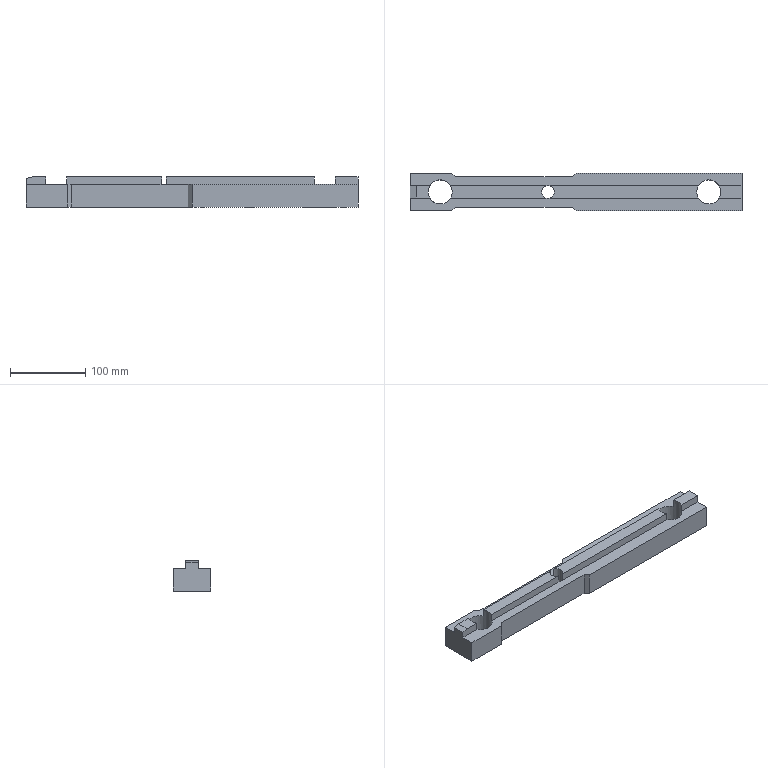Part | STEP file | lll_id3862_x_t | 1 solid | 45 faces | box 440 x 50 x 40 mm | volume 602620 mm3 | plane 31 | cylinder 10 | cone 4 | commonest cylinder face diameters 6.806 x4 11 x2 32 x2 17 x1 22 x1
STEP:
#1=CARTESIAN_POINT('',(2899.856,8.,0.));
#2=VERTEX_POINT('',#1);
#3=CARTESIAN_POINT('',(2899.856,8.,-10.));
#4=VERTEX_POINT('',#3);
#5=CARTESIAN_POINT('',(2899.856,8.,-5.));
#6=DIRECTION('',(0.,0.,-1.));
#7=VECTOR('',#6,1.);
#8=LINE('',#5,#7);
#9=EDGE_CURVE('',#2,#4,#8,.T.);
#10=ORIENTED_EDGE('',*,*,#9,.F.);
#11=CARTESIAN_POINT('',(2930.,8.,0.));
#12=VERTEX_POINT('',#11);
#13=CARTESIAN_POINT('',(2772.5,8.,0.));
#14=DIRECTION('',(1.,0.,0.));
#15=VECTOR('',#14,1.);
#16=LINE('',#13,#15);
#17=EDGE_CURVE('',#2,#12,#16,.T.);
#18=ORIENTED_EDGE('',*,*,#17,.T.);
#19=CARTESIAN_POINT('',(2930.,8.,-10.));
#20=VERTEX_POINT('',#19);
#21=CARTESIAN_POINT('',(2930.,8.,-50.));
#22=DIRECTION('',(0.,0.,1.));
#23=VECTOR('',#22,1.);
#24=LINE('',#21,#23);
#25=EDGE_CURVE('',#20,#12,#24,.T.);
#26=ORIENTED_EDGE('',*,*,#25,.F.);
#27=CARTESIAN_POINT('',(2772.5,8.,-10.));
#28=DIRECTION('',(-1.,0.,0.));
#29=VECTOR('',#28,1.);
#30=LINE('',#27,#29);
#31=EDGE_CURVE('',#20,#4,#30,.T.);
#32=ORIENTED_EDGE('',*,*,#31,.T.);
#33=EDGE_LOOP('',(#10,#18,#26,#32));
#34=FACE_OUTER_BOUND('',#33,.T.);
#35=CARTESIAN_POINT('',(2580.,8.,-25.));
#36=DIRECTION('',(0.,1.,0.));
#37=DIRECTION('',(0.,0.,-1.));
#38=AXIS2_PLACEMENT_3D('',#35,#36,#37);
#39=PLANE('',#38);
#40=ADVANCED_FACE('',(#34),#39,.T.);
#41=CARTESIAN_POINT('',(2872.144,8.,0.));
#42=VERTEX_POINT('',#41);
#43=CARTESIAN_POINT('',(2872.144,-8.,0.));
#44=VERTEX_POINT('',#43);
#45=CARTESIAN_POINT('',(2886.,0.00007614,0.));
#46=DIRECTION('',(0.,0.,1.));
#47=DIRECTION('',(1.,0.,0.));
#48=AXIS2_PLACEMENT_3D('',#45,#46,#47);
#49=CIRCLE('',#48,16.);
#50=EDGE_CURVE('',#42,#44,#49,.T.);
#51=ORIENTED_EDGE('',*,*,#50,.F.);
#52=CARTESIAN_POINT('',(2675.872,8.,0.));
#53=VERTEX_POINT('',#52);
#54=CARTESIAN_POINT('',(2772.5,8.,0.));
#55=DIRECTION('',(1.,0.,0.));
#56=VECTOR('',#55,1.);
#57=LINE('',#54,#56);
#58=EDGE_CURVE('',#53,#42,#57,.T.);
#59=ORIENTED_EDGE('',*,*,#58,.F.);
#60=CARTESIAN_POINT('',(2675.872,-8.,0.));
#61=VERTEX_POINT('',#60);
#62=CARTESIAN_POINT('',(2673.,0.,0.));
#63=DIRECTION('',(0.,0.,1.));
#64=DIRECTION('',(-1.,0.,0.));
#65=AXIS2_PLACEMENT_3D('',#62,#63,#64);
#66=CIRCLE('',#65,8.5);
#67=EDGE_CURVE('',#61,#53,#66,.T.);
#68=ORIENTED_EDGE('',*,*,#67,.F.);
#69=CARTESIAN_POINT('',(2772.5,-8.,0.));
#70=DIRECTION('',(1.,0.,0.));
#71=VECTOR('',#70,1.);
#72=LINE('',#69,#71);
#73=EDGE_CURVE('',#61,#44,#72,.T.);
#74=ORIENTED_EDGE('',*,*,#73,.T.);
#75=EDGE_LOOP('',(#51,#59,#68,#74));
#76=FACE_OUTER_BOUND('',#75,.T.);
#77=CARTESIAN_POINT('',(2772.5,0.00007613,0.));
#78=DIRECTION('',(0.,0.,1.));
#79=DIRECTION('',(1.,0.,0.));
#80=AXIS2_PLACEMENT_3D('',#77,#78,#79);
#81=PLANE('',#80);
#82=ADVANCED_FACE('',(#76),#81,.T.);
#83=CARTESIAN_POINT('',(2872.144,-8.,-10.));
#84=VERTEX_POINT('',#83);
#85=CARTESIAN_POINT('',(2872.144,-8.,-5.));
#86=DIRECTION('',(0.,0.,-1.));
#87=VECTOR('',#86,1.);
#88=LINE('',#85,#87);
#89=EDGE_CURVE('',#44,#84,#88,.T.);
#90=ORIENTED_EDGE('',*,*,#89,.F.);
#91=ORIENTED_EDGE('',*,*,#73,.F.);
#92=CARTESIAN_POINT('',(2675.872,-8.,-10.));
#93=VERTEX_POINT('',#92);
#94=CARTESIAN_POINT('',(2675.872,-8.,2.5));
#95=DIRECTION('',(0.,0.,1.));
#96=VECTOR('',#95,1.);
#97=LINE('',#94,#96);
#98=EDGE_CURVE('',#93,#61,#97,.T.);
#99=ORIENTED_EDGE('',*,*,#98,.F.);
#100=CARTESIAN_POINT('',(2580.,-8.,-10.));
#101=DIRECTION('',(-1.,0.,0.));
#102=VECTOR('',#101,1.);
#103=LINE('',#100,#102);
#104=EDGE_CURVE('',#84,#93,#103,.T.);
#105=ORIENTED_EDGE('',*,*,#104,.F.);
#106=EDGE_LOOP('',(#90,#91,#99,#105));
#107=FACE_OUTER_BOUND('',#106,.T.);
#108=CARTESIAN_POINT('',(2580.,-8.,-25.));
#109=DIRECTION('',(0.,-1.,0.));
#110=DIRECTION('',(0.,0.,1.));
#111=AXIS2_PLACEMENT_3D('',#108,#109,#110);
#112=PLANE('',#111);
#113=ADVANCED_FACE('',(#107),#112,.T.);
#114=CARTESIAN_POINT('',(2863.903,0.00007614,-40.));
#115=VERTEX_POINT('',#114);
#116=CARTESIAN_POINT('',(2860.5,0.00007614,-40.));
#117=DIRECTION('',(0.,0.,1.));
#118=DIRECTION('',(1.,0.,0.));
#119=AXIS2_PLACEMENT_3D('',#116,#117,#118);
#120=CIRCLE('',#119,3.403);
#121=EDGE_CURVE('',#115,#115,#120,.T.);
#122=ORIENTED_EDGE('',*,*,#121,.T.);
#123=EDGE_LOOP('',(#122));
#124=FACE_BOUND('',#123,.T.);
#125=CARTESIAN_POINT('',(2914.903,0.00007614,-40.));
#126=VERTEX_POINT('',#125);
#127=CARTESIAN_POINT('',(2911.5,0.00007614,-40.));
#128=DIRECTION('',(0.,0.,1.));
#129=DIRECTION('',(1.,0.,0.));
#130=AXIS2_PLACEMENT_3D('',#127,#128,#129);
#131=CIRCLE('',#130,3.403);
#132=EDGE_CURVE('',#126,#126,#131,.T.);
#133=ORIENTED_EDGE('',*,*,#132,.T.);
#134=EDGE_LOOP('',(#133));
#135=FACE_BOUND('',#134,.T.);
#136=CARTESIAN_POINT('',(2558.903,0.00007614,-40.));
#137=VERTEX_POINT('',#136);
#138=CARTESIAN_POINT('',(2555.5,0.00007614,-40.));
#139=DIRECTION('',(0.,0.,1.));
#140=DIRECTION('',(1.,0.,0.));
#141=AXIS2_PLACEMENT_3D('',#138,#139,#140);
#142=CIRCLE('',#141,3.403);
#143=EDGE_CURVE('',#137,#137,#142,.T.);
#144=ORIENTED_EDGE('',*,*,#143,.T.);
#145=EDGE_LOOP('',(#144));
#146=FACE_BOUND('',#145,.T.);
#147=CARTESIAN_POINT('',(2507.903,0.00007614,-40.));
#148=VERTEX_POINT('',#147);
#149=CARTESIAN_POINT('',(2504.5,0.00007614,-40.));
#150=DIRECTION('',(0.,0.,1.));
#151=DIRECTION('',(1.,0.,0.));
#152=AXIS2_PLACEMENT_3D('',#149,#150,#151);
#153=CIRCLE('',#152,3.403);
#154=EDGE_CURVE('',#148,#148,#153,.T.);
#155=ORIENTED_EDGE('',*,*,#154,.T.);
#156=EDGE_LOOP('',(#155));
#157=FACE_BOUND('',#156,.T.);
#158=CARTESIAN_POINT('',(2902.,0.00007614,-40.));
#159=VERTEX_POINT('',#158);
#160=CARTESIAN_POINT('',(2886.,0.00007614,-40.));
#161=DIRECTION('',(0.,0.,1.));
#162=DIRECTION('',(1.,0.,0.));
#163=AXIS2_PLACEMENT_3D('',#160,#161,#162);
#164=CIRCLE('',#163,16.);
#165=EDGE_CURVE('',#159,#159,#164,.T.);
#166=ORIENTED_EDGE('',*,*,#165,.T.);
#167=EDGE_LOOP('',(#166));
#168=FACE_BOUND('',#167,.T.);
#169=CARTESIAN_POINT('',(2726.,0.,-40.));
#170=VERTEX_POINT('',#169);
#171=CARTESIAN_POINT('',(2715.,0.,-40.));
#172=DIRECTION('',(0.,0.,1.));
#173=DIRECTION('',(1.,0.,0.));
#174=AXIS2_PLACEMENT_3D('',#171,#172,#173);
#175=CIRCLE('',#174,11.);
#176=EDGE_CURVE('',#170,#170,#175,.T.);
#177=ORIENTED_EDGE('',*,*,#176,.T.);
#178=EDGE_LOOP('',(#177));
#179=FACE_BOUND('',#178,.T.);
#180=CARTESIAN_POINT('',(2550.,-20.,-40.));
#181=VERTEX_POINT('',#180);
#182=CARTESIAN_POINT('',(2705.,-20.,-40.));
#183=VERTEX_POINT('',#182);
#184=CARTESIAN_POINT('',(2507.5,-20.,-40.));
#185=DIRECTION('',(1.,0.,0.));
#186=VECTOR('',#185,1.);
#187=LINE('',#184,#186);
#188=EDGE_CURVE('',#181,#183,#187,.T.);
#189=ORIENTED_EDGE('',*,*,#188,.F.);
#190=CARTESIAN_POINT('',(2545.,-25.,-40.));
#191=VERTEX_POINT('',#190);
#192=CARTESIAN_POINT('',(2550.,-20.,-40.));
#193=DIRECTION('',(-0.7071,-0.7071,0.));
#194=VECTOR('',#193,1.);
#195=LINE('',#192,#194);
#196=EDGE_CURVE('',#181,#191,#195,.T.);
#197=ORIENTED_EDGE('',*,*,#196,.T.);
#198=CARTESIAN_POINT('',(2490.,-25.,-40.));
#199=VERTEX_POINT('',#198);
#200=CARTESIAN_POINT('',(2507.5,-25.,-40.));
#201=DIRECTION('',(1.,0.,0.));
#202=VECTOR('',#201,1.);
#203=LINE('',#200,#202);
#204=EDGE_CURVE('',#199,#191,#203,.T.);
#205=ORIENTED_EDGE('',*,*,#204,.F.);
#206=CARTESIAN_POINT('',(2490.,25.,-40.));
#207=VERTEX_POINT('',#206);
#208=CARTESIAN_POINT('',(2490.,0.00007614,-40.));
#209=DIRECTION('',(0.,-1.,0.));
#210=VECTOR('',#209,1.);
#211=LINE('',#208,#210);
#212=EDGE_CURVE('',#207,#199,#211,.T.);
#213=ORIENTED_EDGE('',*,*,#212,.F.);
#214=CARTESIAN_POINT('',(2545.,25.,-40.));
#215=VERTEX_POINT('',#214);
#216=CARTESIAN_POINT('',(2772.5,25.,-40.));
#217=DIRECTION('',(1.,0.,0.));
#218=VECTOR('',#217,1.);
#219=LINE('',#216,#218);
#220=EDGE_CURVE('',#207,#215,#219,.T.);
#221=ORIENTED_EDGE('',*,*,#220,.T.);
#222=CARTESIAN_POINT('',(2550.,20.,-40.));
#223=VERTEX_POINT('',#222);
#224=CARTESIAN_POINT('',(2545.,25.,-40.));
#225=DIRECTION('',(0.7071,-0.7071,0.));
#226=VECTOR('',#225,1.);
#227=LINE('',#224,#226);
#228=EDGE_CURVE('',#215,#223,#227,.T.);
#229=ORIENTED_EDGE('',*,*,#228,.T.);
#230=CARTESIAN_POINT('',(2705.,20.,-40.));
#231=VERTEX_POINT('',#230);
#232=CARTESIAN_POINT('',(2772.5,20.,-40.));
#233=DIRECTION('',(1.,0.,0.));
#234=VECTOR('',#233,1.);
#235=LINE('',#232,#234);
#236=EDGE_CURVE('',#223,#231,#235,.T.);
#237=ORIENTED_EDGE('',*,*,#236,.T.);
#238=CARTESIAN_POINT('',(2710.,25.,-40.));
#239=VERTEX_POINT('',#238);
#240=CARTESIAN_POINT('',(2710.,25.,-40.));
#241=DIRECTION('',(0.7071,0.7071,0.));
#242=VECTOR('',#241,1.);
#243=LINE('',#240,#242);
#244=EDGE_CURVE('',#231,#239,#243,.T.);
#245=ORIENTED_EDGE('',*,*,#244,.T.);
#246=CARTESIAN_POINT('',(2930.,25.,-40.));
#247=VERTEX_POINT('',#246);
#248=CARTESIAN_POINT('',(2772.5,25.,-40.));
#249=DIRECTION('',(1.,0.,0.));
#250=VECTOR('',#249,1.);
#251=LINE('',#248,#250);
#252=EDGE_CURVE('',#239,#247,#251,.T.);
#253=ORIENTED_EDGE('',*,*,#252,.T.);
#254=CARTESIAN_POINT('',(2930.,-25.,-40.));
#255=VERTEX_POINT('',#254);
#256=CARTESIAN_POINT('',(2930.,0.00007613,-40.));
#257=DIRECTION('',(0.,-1.,0.));
#258=VECTOR('',#257,1.);
#259=LINE('',#256,#258);
#260=EDGE_CURVE('',#247,#255,#259,.T.);
#261=ORIENTED_EDGE('',*,*,#260,.T.);
#262=CARTESIAN_POINT('',(2710.,-25.,-40.));
#263=VERTEX_POINT('',#262);
#264=CARTESIAN_POINT('',(2507.5,-25.,-40.));
#265=DIRECTION('',(1.,0.,0.));
#266=VECTOR('',#265,1.);
#267=LINE('',#264,#266);
#268=EDGE_CURVE('',#263,#255,#267,.T.);
#269=ORIENTED_EDGE('',*,*,#268,.F.);
#270=CARTESIAN_POINT('',(2710.,-25.,-40.));
#271=DIRECTION('',(-0.7071,0.7071,0.));
#272=VECTOR('',#271,1.);
#273=LINE('',#270,#272);
#274=EDGE_CURVE('',#263,#183,#273,.T.);
#275=ORIENTED_EDGE('',*,*,#274,.T.);
#276=EDGE_LOOP('',(#189,#197,#205,#213,#221,#229,#237,#245,#253,#261,#269,#275));
#277=FACE_BOUND('',#276,.T.);
#278=CARTESIAN_POINT('',(2681.5,0.,-40.));
#279=VERTEX_POINT('',#278);
#280=CARTESIAN_POINT('',(2673.,0.,-40.));
#281=DIRECTION('',(0.,0.,1.));
#282=DIRECTION('',(1.,0.,0.));
#283=AXIS2_PLACEMENT_3D('',#280,#281,#282);
#284=CIRCLE('',#283,8.5);
#285=EDGE_CURVE('',#279,#279,#284,.T.);
#286=ORIENTED_EDGE('',*,*,#285,.T.);
#287=EDGE_LOOP('',(#286));
#288=FACE_BOUND('',#287,.T.);
#289=CARTESIAN_POINT('',(2546.,0.00007614,-40.));
#290=VERTEX_POINT('',#289);
#291=CARTESIAN_POINT('',(2530.,0.00007614,-40.));
#292=DIRECTION('',(0.,0.,-1.));
#293=DIRECTION('',(1.,0.,0.));
#294=AXIS2_PLACEMENT_3D('',#291,#292,#293);
#295=CIRCLE('',#294,16.);
#296=EDGE_CURVE('',#290,#290,#295,.T.);
#297=ORIENTED_EDGE('',*,*,#296,.F.);
#298=EDGE_LOOP('',(#297));
#299=FACE_BOUND('',#298,.T.);
#300=CARTESIAN_POINT('',(2632.5,0.00007613,-40.));
#301=VERTEX_POINT('',#300);
#302=CARTESIAN_POINT('',(2627.,0.00007613,-40.));
#303=DIRECTION('',(0.,0.,1.));
#304=DIRECTION('',(1.,0.,0.));
#305=AXIS2_PLACEMENT_3D('',#302,#303,#304);
#306=CIRCLE('',#305,5.5);
#307=EDGE_CURVE('',#301,#301,#306,.T.);
#308=ORIENTED_EDGE('',*,*,#307,.T.);
#309=EDGE_LOOP('',(#308));
#310=FACE_BOUND('',#309,.T.);
#311=CARTESIAN_POINT('',(2792.5,0.00007613,-40.));
#312=VERTEX_POINT('',#311);
#313=CARTESIAN_POINT('',(2787.,0.00007613,-40.));
#314=DIRECTION('',(0.,0.,1.));
#315=DIRECTION('',(1.,0.,0.));
#316=AXIS2_PLACEMENT_3D('',#313,#314,#315);
#317=CIRCLE('',#316,5.5);
#318=EDGE_CURVE('',#312,#312,#317,.T.);
#319=ORIENTED_EDGE('',*,*,#318,.T.);
#320=EDGE_LOOP('',(#319));
#321=FACE_BOUND('',#320,.T.);
#322=CARTESIAN_POINT('',(2507.5,0.00007614,-40.));
#323=DIRECTION('',(0.,0.,1.));
#324=DIRECTION('',(0.,-1.,0.));
#325=AXIS2_PLACEMENT_3D('',#322,#323,#324);
#326=PLANE('',#325);
#327=ADVANCED_FACE('',(#124,#135,#146,#157,#168,#179,#277,#288,#299,#310,#321),#326,.F.);
#328=CARTESIAN_POINT('',(2516.144,-8.,-10.));
#329=VERTEX_POINT('',#328);
#330=CARTESIAN_POINT('',(2543.856,-8.,-10.));
#331=VERTEX_POINT('',#330);
#332=CARTESIAN_POINT('',(2530.,0.00007614,-10.));
#333=DIRECTION('',(0.,0.,1.));
#334=DIRECTION('',(1.,0.,0.));
#335=AXIS2_PLACEMENT_3D('',#332,#333,#334);
#336=CIRCLE('',#335,16.);
#337=EDGE_CURVE('',#329,#331,#336,.T.);
#338=ORIENTED_EDGE('',*,*,#337,.F.);
#339=CARTESIAN_POINT('',(2490.,-8.,-10.));
#340=VERTEX_POINT('',#339);
#341=CARTESIAN_POINT('',(2580.,-8.,-10.));
#342=DIRECTION('',(-1.,0.,0.));
#343=VECTOR('',#342,1.);
#344=LINE('',#341,#343);
#345=EDGE_CURVE('',#329,#340,#344,.T.);
#346=ORIENTED_EDGE('',*,*,#345,.T.);
#347=CARTESIAN_POINT('',(2490.,-25.,-10.));
#348=VERTEX_POINT('',#347);
#349=CARTESIAN_POINT('',(2490.,0.00007613,-10.));
#350=DIRECTION('',(0.,-1.,0.));
#351=VECTOR('',#350,1.);
#352=LINE('',#349,#351);
#353=EDGE_CURVE('',#340,#348,#352,.T.);
#354=ORIENTED_EDGE('',*,*,#353,.T.);
#355=CARTESIAN_POINT('',(2545.,-25.,-10.));
#356=VERTEX_POINT('',#355);
#357=CARTESIAN_POINT('',(2772.5,-25.,-10.));
#358=DIRECTION('',(-1.,0.,0.));
#359=VECTOR('',#358,1.);
#360=LINE('',#357,#359);
#361=EDGE_CURVE('',#356,#348,#360,.T.);
#362=ORIENTED_EDGE('',*,*,#361,.F.);
#363=CARTESIAN_POINT('',(2550.,-20.,-10.));
#364=VERTEX_POINT('',#363);
#365=CARTESIAN_POINT('',(2681.25,111.25,-10.));
#366=DIRECTION('',(0.7071,0.7071,0.));
#367=VECTOR('',#366,1.);
#368=LINE('',#365,#367);
#369=EDGE_CURVE('',#356,#364,#368,.T.);
#370=ORIENTED_EDGE('',*,*,#369,.T.);
#371=CARTESIAN_POINT('',(2705.,-20.,-10.));
#372=VERTEX_POINT('',#371);
#373=CARTESIAN_POINT('',(2772.5,-20.,-10.));
#374=DIRECTION('',(-1.,0.,0.));
#375=VECTOR('',#374,1.);
#376=LINE('',#373,#375);
#377=EDGE_CURVE('',#372,#364,#376,.T.);
#378=ORIENTED_EDGE('',*,*,#377,.F.);
#379=CARTESIAN_POINT('',(2710.,-25.,-10.));
#380=VERTEX_POINT('',#379);
#381=CARTESIAN_POINT('',(2728.75,-43.75,-10.));
#382=DIRECTION('',(0.7071,-0.7071,0.));
#383=VECTOR('',#382,1.);
#384=LINE('',#381,#383);
#385=EDGE_CURVE('',#372,#380,#384,.T.);
#386=ORIENTED_EDGE('',*,*,#385,.T.);
#387=CARTESIAN_POINT('',(2930.,-25.,-10.));
#388=VERTEX_POINT('',#387);
#389=CARTESIAN_POINT('',(2772.5,-25.,-10.));
#390=DIRECTION('',(-1.,0.,0.));
#391=VECTOR('',#390,1.);
#392=LINE('',#389,#391);
#393=EDGE_CURVE('',#388,#380,#392,.T.);
#394=ORIENTED_EDGE('',*,*,#393,.F.);
#395=CARTESIAN_POINT('',(2930.,-8.,-10.));
#396=VERTEX_POINT('',#395);
#397=CARTESIAN_POINT('',(2930.,0.00007613,-10.));
#398=DIRECTION('',(0.,-1.,0.));
#399=VECTOR('',#398,1.);
#400=LINE('',#397,#399);
#401=EDGE_CURVE('',#396,#388,#400,.T.);
#402=ORIENTED_EDGE('',*,*,#401,.F.);
#403=CARTESIAN_POINT('',(2899.856,-8.,-10.));
#404=VERTEX_POINT('',#403);
#405=CARTESIAN_POINT('',(2580.,-8.,-10.));
#406=DIRECTION('',(-1.,0.,0.));
#407=VECTOR('',#406,1.);
#408=LINE('',#405,#407);
#409=EDGE_CURVE('',#396,#404,#408,.T.);
#410=ORIENTED_EDGE('',*,*,#409,.T.);
#411=CARTESIAN_POINT('',(2886.,0.00007614,-10.));
#412=DIRECTION('',(0.,0.,1.));
#413=DIRECTION('',(1.,0.,0.));
#414=AXIS2_PLACEMENT_3D('',#411,#412,#413);
#415=CIRCLE('',#414,16.);
#416=EDGE_CURVE('',#84,#404,#415,.T.);
#417=ORIENTED_EDGE('',*,*,#416,.F.);
#418=ORIENTED_EDGE('',*,*,#104,.T.);
#419=CARTESIAN_POINT('',(2670.128,-8.,-10.));
#420=VERTEX_POINT('',#419);
#421=CARTESIAN_POINT('',(2673.,0.,-10.));
#422=DIRECTION('',(0.,0.,1.));
#423=DIRECTION('',(-1.,0.,0.));
#424=AXIS2_PLACEMENT_3D('',#421,#422,#423);
#425=CIRCLE('',#424,8.5);
#426=EDGE_CURVE('',#420,#93,#425,.T.);
#427=ORIENTED_EDGE('',*,*,#426,.F.);
#428=CARTESIAN_POINT('',(2580.,-8.,-10.));
#429=DIRECTION('',(-1.,0.,0.));
#430=VECTOR('',#429,1.);
#431=LINE('',#428,#430);
#432=EDGE_CURVE('',#420,#331,#431,.T.);
#433=ORIENTED_EDGE('',*,*,#432,.T.);
#434=EDGE_LOOP('',(#338,#346,#354,#362,#370,#378,#386,#394,#402,#410,#417,#418,#427,#433));
#435=FACE_OUTER_BOUND('',#434,.T.);
#436=CARTESIAN_POINT('',(2772.5,0.00007613,-10.));
#437=DIRECTION('',(0.,0.,1.));
#438=DIRECTION('',(1.,0.,0.));
#439=AXIS2_PLACEMENT_3D('',#436,#437,#438);
#440=PLANE('',#439);
#441=ADVANCED_FACE('',(#435),#440,.T.);
#442=CARTESIAN_POINT('',(2516.144,8.,0.));
#443=VERTEX_POINT('',#442);
#444=CARTESIAN_POINT('',(2516.144,-8.,0.));
#445=VERTEX_POINT('',#444);
#446=CARTESIAN_POINT('',(2530.,0.00007614,0.));
#447=DIRECTION('',(0.,0.,1.));
#448=DIRECTION('',(1.,0.,0.));
#449=AXIS2_PLACEMENT_3D('',#446,#447,#448);
#450=CIRCLE('',#449,16.);
#451=EDGE_CURVE('',#443,#445,#450,.T.);
#452=ORIENTED_EDGE('',*,*,#451,.F.);
#453=CARTESIAN_POINT('',(2498.,8.,0.));
#454=VERTEX_POINT('',#453);
#455=CARTESIAN_POINT('',(2772.5,8.,0.));
#456=DIRECTION('',(1.,0.,0.));
#457=VECTOR('',#456,1.);
#458=LINE('',#455,#457);
#459=EDGE_CURVE('',#454,#443,#458,.T.);
#460=ORIENTED_EDGE('',*,*,#459,.F.);
#461=CARTESIAN_POINT('',(2498.,-8.,0.));
#462=VERTEX_POINT('',#461);
#463=CARTESIAN_POINT('',(2498.,0.00007613,0.));
#464=DIRECTION('',(0.,-1.,0.));
#465=VECTOR('',#464,1.);
#466=LINE('',#463,#465);
#467=EDGE_CURVE('',#454,#462,#466,.T.);
#468=ORIENTED_EDGE('',*,*,#467,.T.);
#469=CARTESIAN_POINT('',(2772.5,-8.,0.));
#470=DIRECTION('',(1.,0.,0.));
#471=VECTOR('',#470,1.);
#472=LINE('',#469,#471);
#473=EDGE_CURVE('',#462,#445,#472,.T.);
#474=ORIENTED_EDGE('',*,*,#473,.T.);
#475=EDGE_LOOP('',(#452,#460,#468,#474));
#476=FACE_OUTER_BOUND('',#475,.T.);
#477=CARTESIAN_POINT('',(2772.5,0.00007613,0.));
#478=DIRECTION('',(0.,0.,1.));
#479=DIRECTION('',(1.,0.,0.));
#480=AXIS2_PLACEMENT_3D('',#477,#478,#479);
#481=PLANE('',#480);
#482=ADVANCED_FACE('',(#476),#481,.T.);
#483=CARTESIAN_POINT('',(2516.144,-8.,-40.));
#484=DIRECTION('',(0.,0.,-1.));
#485=VECTOR('',#484,1.);
#486=LINE('',#483,#485);
#487=EDGE_CURVE('',#445,#329,#486,.T.);
#488=ORIENTED_EDGE('',*,*,#487,.F.);
#489=ORIENTED_EDGE('',*,*,#473,.F.);
#490=CARTESIAN_POINT('',(2490.,-8.,-2.));
#491=VERTEX_POINT('',#490);
#492=CARTESIAN_POINT('',(2569.294,-8.,17.824));
#493=DIRECTION('',(-0.9701,0.,-0.2425));
#494=VECTOR('',#493,1.);
#495=LINE('',#492,#494);
#496=EDGE_CURVE('',#462,#491,#495,.T.);
#497=ORIENTED_EDGE('',*,*,#496,.T.);
#498=CARTESIAN_POINT('',(2490.,-8.,-25.));
#499=DIRECTION('',(0.,0.,-1.));
#500=VECTOR('',#499,1.);
#501=LINE('',#498,#500);
#502=EDGE_CURVE('',#491,#340,#501,.T.);
#503=ORIENTED_EDGE('',*,*,#502,.T.);
#504=ORIENTED_EDGE('',*,*,#345,.F.);
#505=EDGE_LOOP('',(#488,#489,#497,#503,#504));
#506=FACE_OUTER_BOUND('',#505,.T.);
#507=CARTESIAN_POINT('',(2580.,-8.,-25.));
#508=DIRECTION('',(0.,-1.,0.));
#509=DIRECTION('',(0.,0.,1.));
#510=AXIS2_PLACEMENT_3D('',#507,#508,#509);
#511=PLANE('',#510);
#512=ADVANCED_FACE('',(#506),#511,.T.);
#513=CARTESIAN_POINT('',(2543.856,8.,0.));
#514=VERTEX_POINT('',#513);
#515=CARTESIAN_POINT('',(2543.856,8.,-10.));
#516=VERTEX_POINT('',#515);
#517=CARTESIAN_POINT('',(2543.856,8.,-40.));
#518=DIRECTION('',(0.,0.,-1.));
#519=VECTOR('',#518,1.);
#520=LINE('',#517,#519);
#521=EDGE_CURVE('',#514,#516,#520,.T.);
#522=ORIENTED_EDGE('',*,*,#521,.F.);
#523=CARTESIAN_POINT('',(2670.128,8.,0.));
#524=VERTEX_POINT('',#523);
#525=CARTESIAN_POINT('',(2772.5,8.,0.));
#526=DIRECTION('',(1.,0.,0.));
#527=VECTOR('',#526,1.);
#528=LINE('',#525,#527);
#529=EDGE_CURVE('',#514,#524,#528,.T.);
#530=ORIENTED_EDGE('',*,*,#529,.T.);
#531=CARTESIAN_POINT('',(2670.128,8.,-10.));
#532=VERTEX_POINT('',#531);
#533=CARTESIAN_POINT('',(2670.128,8.,2.5));
#534=DIRECTION('',(0.,0.,1.));
#535=VECTOR('',#534,1.);
#536=LINE('',#533,#535);
#537=EDGE_CURVE('',#532,#524,#536,.T.);
#538=ORIENTED_EDGE('',*,*,#537,.F.);
#539=CARTESIAN_POINT('',(2772.5,8.,-10.));
#540=DIRECTION('',(-1.,0.,0.));
#541=VECTOR('',#540,1.);
#542=LINE('',#539,#541);
#543=EDGE_CURVE('',#532,#516,#542,.T.);
#544=ORIENTED_EDGE('',*,*,#543,.T.);
#545=EDGE_LOOP('',(#522,#530,#538,#544));
#546=FACE_OUTER_BOUND('',#545,.T.);
#547=CARTESIAN_POINT('',(2580.,8.,-25.));
#548=DIRECTION('',(0.,1.,0.));
#549=DIRECTION('',(0.,0.,-1.));
#550=AXIS2_PLACEMENT_3D('',#547,#548,#549);
#551=PLANE('',#550);
#552=ADVANCED_FACE('',(#546),#551,.T.);
#553=ORIENTED_EDGE('',*,*,#393,.T.);
#554=CARTESIAN_POINT('',(2710.,-25.,-50.));
#555=DIRECTION('',(0.,0.,-1.));
#556=VECTOR('',#555,1.);
#557=LINE('',#554,#556);
#558=EDGE_CURVE('',#380,#263,#557,.T.);
#559=ORIENTED_EDGE('',*,*,#558,.T.);
#560=ORIENTED_EDGE('',*,*,#268,.T.);
#561=CARTESIAN_POINT('',(2930.,-25.,-50.));
#562=DIRECTION('',(0.,0.,1.));
#563=VECTOR('',#562,1.);
#564=LINE('',#561,#563);
#565=EDGE_CURVE('',#255,#388,#564,.T.);
#566=ORIENTED_EDGE('',*,*,#565,.T.);
#567=EDGE_LOOP('',(#553,#559,#560,#566));
#568=FACE_OUTER_BOUND('',#567,.T.);
#569=CARTESIAN_POINT('',(2772.5,-25.,-50.));
#570=DIRECTION('',(0.,-1.,0.));
#571=DIRECTION('',(0.,0.,-1.));
#572=AXIS2_PLACEMENT_3D('',#569,#570,#571);
#573=PLANE('',#572);
#574=ADVANCED_FACE('',(#568),#573,.T.);
#575=CARTESIAN_POINT('',(2516.144,8.,-10.));
#576=VERTEX_POINT('',#575);
#577=CARTESIAN_POINT('',(2530.,0.00007614,-10.));
#578=DIRECTION('',(0.,0.,1.));
#579=DIRECTION('',(1.,0.,0.));
#580=AXIS2_PLACEMENT_3D('',#577,#578,#579);
#581=CIRCLE('',#580,16.);
#582=EDGE_CURVE('',#516,#576,#581,.T.);
#583=ORIENTED_EDGE('',*,*,#582,.F.);
#584=ORIENTED_EDGE('',*,*,#543,.F.);
#585=CARTESIAN_POINT('',(2675.872,8.,-10.));
#586=VERTEX_POINT('',#585);
#587=CARTESIAN_POINT('',(2673.,0.,-10.));
#588=DIRECTION('',(0.,0.,1.));
#589=DIRECTION('',(-1.,0.,0.));
#590=AXIS2_PLACEMENT_3D('',#587,#588,#589);
#591=CIRCLE('',#590,8.5);
#592=EDGE_CURVE('',#586,#532,#591,.T.);
#593=ORIENTED_EDGE('',*,*,#592,.F.);
#594=CARTESIAN_POINT('',(2872.144,8.,-10.));
#595=VERTEX_POINT('',#594);
#596=CARTESIAN_POINT('',(2772.5,8.,-10.));
#597=DIRECTION('',(-1.,0.,0.));
#598=VECTOR('',#597,1.);
#599=LINE('',#596,#598);
#600=EDGE_CURVE('',#595,#586,#599,.T.);
#601=ORIENTED_EDGE('',*,*,#600,.F.);
#602=CARTESIAN_POINT('',(2886.,0.00007614,-10.));
#603=DIRECTION('',(0.,0.,1.));
#604=DIRECTION('',(1.,0.,0.));
#605=AXIS2_PLACEMENT_3D('',#602,#603,#604);
#606=CIRCLE('',#605,16.);
#607=EDGE_CURVE('',#4,#595,#606,.T.);
#608=ORIENTED_EDGE('',*,*,#607,.F.);
#609=ORIENTED_EDGE('',*,*,#31,.F.);
#610=CARTESIAN_POINT('',(2930.,25.,-10.));
#611=VERTEX_POINT('',#610);
#612=CARTESIAN_POINT('',(2930.,0.00007613,-10.));
#613=DIRECTION('',(0.,-1.,0.));
#614=VECTOR('',#613,1.);
#615=LINE('',#612,#614);
#616=EDGE_CURVE('',#611,#20,#615,.T.);
#617=ORIENTED_EDGE('',*,*,#616,.F.);
#618=CARTESIAN_POINT('',(2710.,25.,-10.));
#619=VERTEX_POINT('',#618);
#620=CARTESIAN_POINT('',(2772.5,25.,-10.));
#621=DIRECTION('',(1.,0.,0.));
#622=VECTOR('',#621,1.);
#623=LINE('',#620,#622);
#624=EDGE_CURVE('',#619,#611,#623,.T.);
#625=ORIENTED_EDGE('',*,*,#624,.F.);
#626=CARTESIAN_POINT('',(2705.,20.,-10.));
#627=VERTEX_POINT('',#626);
#628=CARTESIAN_POINT('',(2728.75,43.75,-10.));
#629=DIRECTION('',(-0.7071,-0.7071,0.));
#630=VECTOR('',#629,1.);
#631=LINE('',#628,#630);
#632=EDGE_CURVE('',#619,#627,#631,.T.);
#633=ORIENTED_EDGE('',*,*,#632,.T.);
#634=CARTESIAN_POINT('',(2550.,20.,-10.));
#635=VERTEX_POINT('',#634);
#636=CARTESIAN_POINT('',(2772.5,20.,-10.));
#637=DIRECTION('',(1.,0.,0.));
#638=VECTOR('',#637,1.);
#639=LINE('',#636,#638);
#640=EDGE_CURVE('',#635,#627,#639,.T.);
#641=ORIENTED_EDGE('',*,*,#640,.F.);
#642=CARTESIAN_POINT('',(2545.,25.,-10.));
#643=VERTEX_POINT('',#642);
#644=CARTESIAN_POINT('',(2681.25,-111.25,-10.));
#645=DIRECTION('',(-0.7071,0.7071,0.));
#646=VECTOR('',#645,1.);
#647=LINE('',#644,#646);
#648=EDGE_CURVE('',#635,#643,#647,.T.);
#649=ORIENTED_EDGE('',*,*,#648,.T.);
#650=CARTESIAN_POINT('',(2490.,25.,-10.));
#651=VERTEX_POINT('',#650);
#652=CARTESIAN_POINT('',(2772.5,25.,-10.));
#653=DIRECTION('',(1.,0.,0.));
#654=VECTOR('',#653,1.);
#655=LINE('',#652,#654);
#656=EDGE_CURVE('',#651,#643,#655,.T.);
#657=ORIENTED_EDGE('',*,*,#656,.F.);
#658=CARTESIAN_POINT('',(2490.,8.,-10.));
#659=VERTEX_POINT('',#658);
#660=CARTESIAN_POINT('',(2490.,0.00007613,-10.));
#661=DIRECTION('',(0.,-1.,0.));
#662=VECTOR('',#661,1.);
#663=LINE('',#660,#662);
#664=EDGE_CURVE('',#651,#659,#663,.T.);
#665=ORIENTED_EDGE('',*,*,#664,.T.);
#666=CARTESIAN_POINT('',(2772.5,8.,-10.));
#667=DIRECTION('',(-1.,0.,0.));
#668=VECTOR('',#667,1.);
#669=LINE('',#666,#668);
#670=EDGE_CURVE('',#576,#659,#669,.T.);
#671=ORIENTED_EDGE('',*,*,#670,.F.);
#672=EDGE_LOOP('',(#583,#584,#593,#601,#608,#609,#617,#625,#633,#641,#649,#657,#665,#671));
#673=FACE_OUTER_BOUND('',#672,.T.);
#674=CARTESIAN_POINT('',(2772.5,0.00007613,-10.));
#675=DIRECTION('',(0.,0.,1.));
#676=DIRECTION('',(1.,0.,0.));
#677=AXIS2_PLACEMENT_3D('',#674,#675,#676);
#678=PLANE('',#677);
#679=ADVANCED_FACE('',(#673),#678,.T.);
#680=ORIENTED_EDGE('',*,*,#252,.F.);
#681=CARTESIAN_POINT('',(2710.,25.,-50.));
#682=DIRECTION('',(0.,0.,1.));
#683=VECTOR('',#682,1.);
#684=LINE('',#681,#683);
#685=EDGE_CURVE('',#239,#619,#684,.T.);
#686=ORIENTED_EDGE('',*,*,#685,.T.);
#687=ORIENTED_EDGE('',*,*,#624,.T.);
#688=CARTESIAN_POINT('',(2930.,25.,-50.));
#689=DIRECTION('',(0.,0.,1.));
#690=VECTOR('',#689,1.);
#691=LINE('',#688,#690);
#692=EDGE_CURVE('',#247,#611,#691,.T.);
#693=ORIENTED_EDGE('',*,*,#692,.F.);
#694=EDGE_LOOP('',(#680,#686,#687,#693));
#695=FACE_OUTER_BOUND('',#694,.T.);
#696=CARTESIAN_POINT('',(2772.5,25.,-50.));
#697=DIRECTION('',(0.,1.,0.));
#698=DIRECTION('',(0.,0.,1.));
#699=AXIS2_PLACEMENT_3D('',#696,#697,#698);
#700=PLANE('',#699);
#701=ADVANCED_FACE('',(#695),#700,.T.);
#702=CARTESIAN_POINT('',(2872.144,8.,-5.));
#703=DIRECTION('',(0.,0.,1.));
#704=VECTOR('',#703,1.);
#705=LINE('',#702,#704);
#706=EDGE_CURVE('',#595,#42,#705,.T.);
#707=ORIENTED_EDGE('',*,*,#706,.F.);
#708=ORIENTED_EDGE('',*,*,#600,.T.);
#709=CARTESIAN_POINT('',(2675.872,8.,2.5));
#710=DIRECTION('',(0.,0.,-1.));
#711=VECTOR('',#710,1.);
#712=LINE('',#709,#711);
#713=EDGE_CURVE('',#53,#586,#712,.T.);
#714=ORIENTED_EDGE('',*,*,#713,.F.);
#715=ORIENTED_EDGE('',*,*,#58,.T.);
#716=EDGE_LOOP('',(#707,#708,#714,#715));
#717=FACE_OUTER_BOUND('',#716,.T.);
#718=CARTESIAN_POINT('',(2580.,8.,-25.));
#719=DIRECTION('',(0.,1.,0.));
#720=DIRECTION('',(0.,0.,-1.));
#721=AXIS2_PLACEMENT_3D('',#718,#719,#720);
#722=PLANE('',#721);
#723=ADVANCED_FACE('',(#717),#722,.T.);
#724=CARTESIAN_POINT('',(2899.856,-8.,0.));
#725=VERTEX_POINT('',#724);
#726=CARTESIAN_POINT('',(2886.,0.00007614,0.));
#727=DIRECTION('',(0.,0.,1.));
#728=DIRECTION('',(1.,0.,0.));
#729=AXIS2_PLACEMENT_3D('',#726,#727,#728);
#730=CIRCLE('',#729,16.);
#731=EDGE_CURVE('',#725,#2,#730,.T.);
#732=ORIENTED_EDGE('',*,*,#731,.F.);
#733=CARTESIAN_POINT('',(2930.,-8.,0.));
#734=VERTEX_POINT('',#733);
#735=CARTESIAN_POINT('',(2772.5,-8.,0.));
#736=DIRECTION('',(1.,0.,0.));
#737=VECTOR('',#736,1.);
#738=LINE('',#735,#737);
#739=EDGE_CURVE('',#725,#734,#738,.T.);
#740=ORIENTED_EDGE('',*,*,#739,.T.);
#741=CARTESIAN_POINT('',(2930.,0.00007613,0.));
#742=DIRECTION('',(0.,-1.,0.));
#743=VECTOR('',#742,1.);
#744=LINE('',#741,#743);
#745=EDGE_CURVE('',#12,#734,#744,.T.);
#746=ORIENTED_EDGE('',*,*,#745,.F.);
#747=ORIENTED_EDGE('',*,*,#17,.F.);
#748=EDGE_LOOP('',(#732,#740,#746,#747));
#749=FACE_OUTER_BOUND('',#748,.T.);
#750=CARTESIAN_POINT('',(2772.5,0.00007613,0.));
#751=DIRECTION('',(0.,0.,1.));
#752=DIRECTION('',(1.,0.,0.));
#753=AXIS2_PLACEMENT_3D('',#750,#751,#752);
#754=PLANE('',#753);
#755=ADVANCED_FACE('',(#749),#754,.T.);
#756=CARTESIAN_POINT('',(2899.856,-8.,-5.));
#757=DIRECTION('',(0.,0.,1.));
#758=VECTOR('',#757,1.);
#759=LINE('',#756,#758);
#760=EDGE_CURVE('',#404,#725,#759,.T.);
#761=ORIENTED_EDGE('',*,*,#760,.F.);
#762=ORIENTED_EDGE('',*,*,#409,.F.);
#763=CARTESIAN_POINT('',(2930.,-8.,-50.));
#764=DIRECTION('',(0.,0.,1.));
#765=VECTOR('',#764,1.);
#766=LINE('',#763,#765);
#767=EDGE_CURVE('',#396,#734,#766,.T.);
#768=ORIENTED_EDGE('',*,*,#767,.T.);
#769=ORIENTED_EDGE('',*,*,#739,.F.);
#770=EDGE_LOOP('',(#761,#762,#768,#769));
#771=FACE_OUTER_BOUND('',#770,.T.);
#772=CARTESIAN_POINT('',(2580.,-8.,-25.));
#773=DIRECTION('',(0.,-1.,0.));
#774=DIRECTION('',(0.,0.,1.));
#775=AXIS2_PLACEMENT_3D('',#772,#773,#774);
#776=PLANE('',#775);
#777=ADVANCED_FACE('',(#771),#776,.T.);
#778=ORIENTED_EDGE('',*,*,#565,.F.);
#779=ORIENTED_EDGE('',*,*,#260,.F.);
#780=ORIENTED_EDGE('',*,*,#692,.T.);
#781=ORIENTED_EDGE('',*,*,#616,.T.);
#782=ORIENTED_EDGE('',*,*,#25,.T.);
#783=ORIENTED_EDGE('',*,*,#745,.T.);
#784=ORIENTED_EDGE('',*,*,#767,.F.);
#785=ORIENTED_EDGE('',*,*,#401,.T.);
#786=EDGE_LOOP('',(#778,#779,#780,#781,#782,#783,#784,#785));
#787=FACE_OUTER_BOUND('',#786,.T.);
#788=CARTESIAN_POINT('',(2930.,0.00007613,-50.));
#789=DIRECTION('',(1.,0.,0.));
#790=DIRECTION('',(0.,0.,-1.));
#791=AXIS2_PLACEMENT_3D('',#788,#789,#790);
#792=PLANE('',#791);
#793=ADVANCED_FACE('',(#787),#792,.T.);
#794=CARTESIAN_POINT('',(2704.,0.,-27.));
#795=VERTEX_POINT('',#794);
#796=CARTESIAN_POINT('',(2715.,0.,-27.));
#797=DIRECTION('',(0.,0.,1.));
#798=DIRECTION('',(-1.,0.,0.));
#799=AXIS2_PLACEMENT_3D('',#796,#797,#798);
#800=CIRCLE('',#799,11.);
#801=EDGE_CURVE('',#795,#795,#800,.T.);
#802=ORIENTED_EDGE('',*,*,#801,.T.);
#803=EDGE_LOOP('',(#802));
#804=FACE_BOUND('',#803,.T.);
#805=ORIENTED_EDGE('',*,*,#176,.F.);
#806=EDGE_LOOP('',(#805));
#807=FACE_BOUND('',#806,.T.);
#808=CARTESIAN_POINT('',(2715.,0.,-27.));
#809=DIRECTION('',(0.,0.,-1.));
#810=DIRECTION('',(-1.,0.,0.));
#811=AXIS2_PLACEMENT_3D('',#808,#809,#810);
#812=CYLINDRICAL_SURFACE('',#811,11.);
#813=ADVANCED_FACE('',(#804,#807),#812,.F.);
#814=ORIENTED_EDGE('',*,*,#801,.F.);
#815=EDGE_LOOP('',(#814));
#816=FACE_OUTER_BOUND('',#815,.T.);
#817=CARTESIAN_POINT('',(2715.,0.,-27.));
#818=DIRECTION('',(0.,0.,1.));
#819=DIRECTION('',(-1.,0.,0.));
#820=AXIS2_PLACEMENT_3D('',#817,#818,#819);
#821=PLANE('',#820);
#822=ADVANCED_FACE('',(#816),#821,.F.);
#823=CARTESIAN_POINT('',(2543.856,-8.,0.));
#824=VERTEX_POINT('',#823);
#825=CARTESIAN_POINT('',(2530.,0.00007614,0.));
#826=DIRECTION('',(0.,0.,1.));
#827=DIRECTION('',(1.,0.,0.));
#828=AXIS2_PLACEMENT_3D('',#825,#826,#827);
#829=CIRCLE('',#828,16.);
#830=EDGE_CURVE('',#824,#514,#829,.T.);
#831=ORIENTED_EDGE('',*,*,#830,.F.);
#832=CARTESIAN_POINT('',(2670.128,-8.,0.));
#833=VERTEX_POINT('',#832);
#834=CARTESIAN_POINT('',(2772.5,-8.,0.));
#835=DIRECTION('',(1.,0.,0.));
#836=VECTOR('',#835,1.);
#837=LINE('',#834,#836);
#838=EDGE_CURVE('',#824,#833,#837,.T.);
#839=ORIENTED_EDGE('',*,*,#838,.T.);
#840=CARTESIAN_POINT('',(2673.,0.,0.));
#841=DIRECTION('',(0.,0.,1.));
#842=DIRECTION('',(-1.,0.,0.));
#843=AXIS2_PLACEMENT_3D('',#840,#841,#842);
#844=CIRCLE('',#843,8.5);
#845=EDGE_CURVE('',#524,#833,#844,.T.);
#846=ORIENTED_EDGE('',*,*,#845,.F.);
#847=ORIENTED_EDGE('',*,*,#529,.F.);
#848=EDGE_LOOP('',(#831,#839,#846,#847));
#849=FACE_OUTER_BOUND('',#848,.T.);
#850=CARTESIAN_POINT('',(2772.5,0.00007613,0.));
#851=DIRECTION('',(0.,0.,1.));
#852=DIRECTION('',(1.,0.,0.));
#853=AXIS2_PLACEMENT_3D('',#850,#851,#852);
#854=PLANE('',#853);
#855=ADVANCED_FACE('',(#849),#854,.T.);
#856=CARTESIAN_POINT('',(2543.856,-8.,-40.));
#857=DIRECTION('',(0.,0.,1.));
#858=VECTOR('',#857,1.);
#859=LINE('',#856,#858);
#860=EDGE_CURVE('',#331,#824,#859,.T.);
#861=ORIENTED_EDGE('',*,*,#860,.F.);
#862=ORIENTED_EDGE('',*,*,#432,.F.);
#863=CARTESIAN_POINT('',(2670.128,-8.,2.5));
#864=DIRECTION('',(0.,0.,-1.));
#865=VECTOR('',#864,1.);
#866=LINE('',#863,#865);
#867=EDGE_CURVE('',#833,#420,#866,.T.);
#868=ORIENTED_EDGE('',*,*,#867,.F.);
#869=ORIENTED_EDGE('',*,*,#838,.F.);
#870=EDGE_LOOP('',(#861,#862,#868,#869));
#871=FACE_OUTER_BOUND('',#870,.T.);
#872=CARTESIAN_POINT('',(2580.,-8.,-25.));
#873=DIRECTION('',(0.,-1.,0.));
#874=DIRECTION('',(0.,0.,1.));
#875=AXIS2_PLACEMENT_3D('',#872,#873,#874);
#876=PLANE('',#875);
#877=ADVANCED_FACE('',(#871),#876,.T.);
#878=CARTESIAN_POINT('',(2516.144,8.,-40.));
#879=DIRECTION('',(0.,0.,1.));
#880=VECTOR('',#879,1.);
#881=LINE('',#878,#880);
#882=EDGE_CURVE('',#576,#443,#881,.T.);
#883=ORIENTED_EDGE('',*,*,#882,.F.);
#884=ORIENTED_EDGE('',*,*,#670,.T.);
#885=CARTESIAN_POINT('',(2490.,8.,-2.));
#886=VERTEX_POINT('',#885);
#887=CARTESIAN_POINT('',(2490.,8.,-25.));
#888=DIRECTION('',(0.,0.,1.));
#889=VECTOR('',#888,1.);
#890=LINE('',#887,#889);
#891=EDGE_CURVE('',#659,#886,#890,.T.);
#892=ORIENTED_EDGE('',*,*,#891,.T.);
#893=CARTESIAN_POINT('',(2569.294,8.,17.824));
#894=DIRECTION('',(0.9701,0.,0.2425));
#895=VECTOR('',#894,1.);
#896=LINE('',#893,#895);
#897=EDGE_CURVE('',#886,#454,#896,.T.);
#898=ORIENTED_EDGE('',*,*,#897,.T.);
#899=ORIENTED_EDGE('',*,*,#459,.T.);
#900=EDGE_LOOP('',(#883,#884,#892,#898,#899));
#901=FACE_OUTER_BOUND('',#900,.T.);
#902=CARTESIAN_POINT('',(2580.,8.,-25.));
#903=DIRECTION('',(0.,1.,0.));
#904=DIRECTION('',(0.,0.,-1.));
#905=AXIS2_PLACEMENT_3D('',#902,#903,#904);
#906=PLANE('',#905);
#907=ADVANCED_FACE('',(#901),#906,.T.);
#908=ORIENTED_EDGE('',*,*,#426,.T.);
#909=ORIENTED_EDGE('',*,*,#98,.T.);
#910=ORIENTED_EDGE('',*,*,#67,.T.);
#911=ORIENTED_EDGE('',*,*,#713,.T.);
#912=ORIENTED_EDGE('',*,*,#592,.T.);
#913=ORIENTED_EDGE('',*,*,#537,.T.);
#914=ORIENTED_EDGE('',*,*,#845,.T.);
#915=ORIENTED_EDGE('',*,*,#867,.T.);
#916=EDGE_LOOP('',(#908,#909,#910,#911,#912,#913,#914,#915));
#917=FACE_BOUND('',#916,.T.);
#918=ORIENTED_EDGE('',*,*,#285,.F.);
#919=EDGE_LOOP('',(#918));
#920=FACE_BOUND('',#919,.T.);
#921=CARTESIAN_POINT('',(2673.,0.,2.5));
#922=DIRECTION('',(0.,0.,-1.));
#923=DIRECTION('',(-1.,0.,0.));
#924=AXIS2_PLACEMENT_3D('',#921,#922,#923);
#925=CYLINDRICAL_SURFACE('',#924,8.5);
#926=ADVANCED_FACE('',(#917,#920),#925,.F.);
#927=CARTESIAN_POINT('',(2705.,20.,-50.));
#928=DIRECTION('',(0.,0.,-1.));
#929=VECTOR('',#928,1.);
#930=LINE('',#927,#929);
#931=EDGE_CURVE('',#627,#231,#930,.T.);
#932=ORIENTED_EDGE('',*,*,#931,.T.);
#933=ORIENTED_EDGE('',*,*,#236,.F.);
#934=CARTESIAN_POINT('',(2550.,20.,-50.));
#935=DIRECTION('',(0.,0.,1.));
#936=VECTOR('',#935,1.);
#937=LINE('',#934,#936);
#938=EDGE_CURVE('',#223,#635,#937,.T.);
#939=ORIENTED_EDGE('',*,*,#938,.T.);
#940=ORIENTED_EDGE('',*,*,#640,.T.);
#941=EDGE_LOOP('',(#932,#933,#939,#940));
#942=FACE_OUTER_BOUND('',#941,.T.);
#943=CARTESIAN_POINT('',(2772.5,20.,-50.));
#944=DIRECTION('',(0.,1.,0.));
#945=DIRECTION('',(0.,0.,1.));
#946=AXIS2_PLACEMENT_3D('',#943,#944,#945);
#947=PLANE('',#946);
#948=ADVANCED_FACE('',(#942),#947,.T.);
#949=CARTESIAN_POINT('',(2705.,-20.,-50.));
#950=DIRECTION('',(0.,0.,1.));
#951=VECTOR('',#950,1.);
#952=LINE('',#949,#951);
#953=EDGE_CURVE('',#183,#372,#952,.T.);
#954=ORIENTED_EDGE('',*,*,#953,.T.);
#955=ORIENTED_EDGE('',*,*,#377,.T.);
#956=CARTESIAN_POINT('',(2550.,-20.,-50.));
#957=DIRECTION('',(0.,0.,1.));
#958=VECTOR('',#957,1.);
#959=LINE('',#956,#958);
#960=EDGE_CURVE('',#181,#364,#959,.T.);
#961=ORIENTED_EDGE('',*,*,#960,.F.);
#962=ORIENTED_EDGE('',*,*,#188,.T.);
#963=EDGE_LOOP('',(#954,#955,#961,#962));
#964=FACE_OUTER_BOUND('',#963,.T.);
#965=CARTESIAN_POINT('',(2772.5,-20.,-50.));
#966=DIRECTION('',(0.,-1.,0.));
#967=DIRECTION('',(0.,0.,-1.));
#968=AXIS2_PLACEMENT_3D('',#965,#966,#967);
#969=PLANE('',#968);
#970=ADVANCED_FACE('',(#964),#969,.T.);
#971=ORIENTED_EDGE('',*,*,#502,.F.);
#972=CARTESIAN_POINT('',(2490.,20.,-2.));
#973=DIRECTION('',(0.,1.,0.));
#974=VECTOR('',#973,1.);
#975=LINE('',#972,#974);
#976=EDGE_CURVE('',#491,#886,#975,.T.);
#977=ORIENTED_EDGE('',*,*,#976,.T.);
#978=ORIENTED_EDGE('',*,*,#891,.F.);
#979=ORIENTED_EDGE('',*,*,#664,.F.);
#980=CARTESIAN_POINT('',(2490.,25.,-50.));
#981=DIRECTION('',(0.,0.,1.));
#982=VECTOR('',#981,1.);
#983=LINE('',#980,#982);
#984=EDGE_CURVE('',#207,#651,#983,.T.);
#985=ORIENTED_EDGE('',*,*,#984,.F.);
#986=ORIENTED_EDGE('',*,*,#212,.T.);
#987=CARTESIAN_POINT('',(2490.,-25.,-35.));
#988=DIRECTION('',(0.,0.,1.));
#989=VECTOR('',#988,1.);
#990=LINE('',#987,#989);
#991=EDGE_CURVE('',#199,#348,#990,.T.);
#992=ORIENTED_EDGE('',*,*,#991,.T.);
#993=ORIENTED_EDGE('',*,*,#353,.F.);
#994=EDGE_LOOP('',(#971,#977,#978,#979,#985,#986,#992,#993));
#995=FACE_OUTER_BOUND('',#994,.T.);
#996=CARTESIAN_POINT('',(2490.,20.,-35.));
#997=DIRECTION('',(-1.,0.,0.));
#998=DIRECTION('',(0.,0.,-1.));
#999=AXIS2_PLACEMENT_3D('',#996,#997,#998);
#1000=PLANE('',#999);
#1001=ADVANCED_FACE('',(#995),#1000,.T.);
#1002=ORIENTED_EDGE('',*,*,#656,.T.);
#1003=CARTESIAN_POINT('',(2545.,25.,-40.));
#1004=DIRECTION('',(0.,0.,-1.));
#1005=VECTOR('',#1004,1.);
#1006=LINE('',#1003,#1005);
#1007=EDGE_CURVE('',#643,#215,#1006,.T.);
#1008=ORIENTED_EDGE('',*,*,#1007,.T.);
#1009=ORIENTED_EDGE('',*,*,#220,.F.);
#1010=ORIENTED_EDGE('',*,*,#984,.T.);
#1011=EDGE_LOOP('',(#1002,#1008,#1009,#1010));
#1012=FACE_OUTER_BOUND('',#1011,.T.);
#1013=CARTESIAN_POINT('',(2772.5,25.,-50.));
#1014=DIRECTION('',(0.,1.,0.));
#1015=DIRECTION('',(0.,0.,1.));
#1016=AXIS2_PLACEMENT_3D('',#1013,#1014,#1015);
#1017=PLANE('',#1016);
#1018=ADVANCED_FACE('',(#1012),#1017,.T.);
#1019=ORIENTED_EDGE('',*,*,#204,.T.);
#1020=CARTESIAN_POINT('',(2545.,-25.,-10.));
#1021=DIRECTION('',(0.,0.,1.));
#1022=VECTOR('',#1021,1.);
#1023=LINE('',#1020,#1022);
#1024=EDGE_CURVE('',#191,#356,#1023,.T.);
#1025=ORIENTED_EDGE('',*,*,#1024,.T.);
#1026=ORIENTED_EDGE('',*,*,#361,.T.);
#1027=ORIENTED_EDGE('',*,*,#991,.F.);
#1028=EDGE_LOOP('',(#1019,#1025,#1026,#1027));
#1029=FACE_OUTER_BOUND('',#1028,.T.);
#1030=CARTESIAN_POINT('',(2772.5,-25.,-50.));
#1031=DIRECTION('',(0.,-1.,0.));
#1032=DIRECTION('',(0.,0.,-1.));
#1033=AXIS2_PLACEMENT_3D('',#1030,#1031,#1032);
#1034=PLANE('',#1033);
#1035=ADVANCED_FACE('',(#1029),#1034,.T.);
#1036=ORIENTED_EDGE('',*,*,#296,.T.);
#1037=EDGE_LOOP('',(#1036));
#1038=FACE_BOUND('',#1037,.T.);
#1039=ORIENTED_EDGE('',*,*,#860,.T.);
#1040=ORIENTED_EDGE('',*,*,#830,.T.);
#1041=ORIENTED_EDGE('',*,*,#521,.T.);
#1042=ORIENTED_EDGE('',*,*,#582,.T.);
#1043=ORIENTED_EDGE('',*,*,#882,.T.);
#1044=ORIENTED_EDGE('',*,*,#451,.T.);
#1045=ORIENTED_EDGE('',*,*,#487,.T.);
#1046=ORIENTED_EDGE('',*,*,#337,.T.);
#1047=EDGE_LOOP('',(#1039,#1040,#1041,#1042,#1043,#1044,#1045,#1046));
#1048=FACE_BOUND('',#1047,.T.);
#1049=CARTESIAN_POINT('',(2530.,0.00007614,-18.));
#1050=DIRECTION('',(0.,0.,1.));
#1051=DIRECTION('',(0.866,-0.5,0.));
#1052=AXIS2_PLACEMENT_3D('',#1049,#1050,#1051);
#1053=CYLINDRICAL_SURFACE('',#1052,16.);
#1054=ADVANCED_FACE('',(#1038,#1048),#1053,.F.);
#1055=ORIENTED_EDGE('',*,*,#706,.T.);
#1056=ORIENTED_EDGE('',*,*,#50,.T.);
#1057=ORIENTED_EDGE('',*,*,#89,.T.);
#1058=ORIENTED_EDGE('',*,*,#416,.T.);
#1059=ORIENTED_EDGE('',*,*,#760,.T.);
#1060=ORIENTED_EDGE('',*,*,#731,.T.);
#1061=ORIENTED_EDGE('',*,*,#9,.T.);
#1062=ORIENTED_EDGE('',*,*,#607,.T.);
#1063=EDGE_LOOP('',(#1055,#1056,#1057,#1058,#1059,#1060,#1061,#1062));
#1064=FACE_BOUND('',#1063,.T.);
#1065=ORIENTED_EDGE('',*,*,#165,.F.);
#1066=EDGE_LOOP('',(#1065));
#1067=FACE_BOUND('',#1066,.T.);
#1068=CARTESIAN_POINT('',(2886.,0.00007614,190.));
#1069=DIRECTION('',(0.,0.,-1.));
#1070=DIRECTION('',(-1.,0.,0.));
#1071=AXIS2_PLACEMENT_3D('',#1068,#1069,#1070);
#1072=CYLINDRICAL_SURFACE('',#1071,16.);
#1073=ADVANCED_FACE('',(#1064,#1067),#1072,.F.);
#1074=ORIENTED_EDGE('',*,*,#897,.F.);
#1075=ORIENTED_EDGE('',*,*,#976,.F.);
#1076=ORIENTED_EDGE('',*,*,#496,.F.);
#1077=ORIENTED_EDGE('',*,*,#467,.F.);
#1078=EDGE_LOOP('',(#1074,#1075,#1076,#1077));
#1079=FACE_OUTER_BOUND('',#1078,.T.);
#1080=CARTESIAN_POINT('',(2498.,0.00007613,0.));
#1081=DIRECTION('',(0.2425,0.,-0.9701));
#1082=DIRECTION('',(0.,-1.,0.));
#1083=AXIS2_PLACEMENT_3D('',#1080,#1081,#1082);
#1084=PLANE('',#1083);
#1085=ADVANCED_FACE('',(#1079),#1084,.F.);
#1086=CARTESIAN_POINT('',(2632.5,0.00007613,-20.));
#1087=VERTEX_POINT('',#1086);
#1088=CARTESIAN_POINT('',(2627.,0.00007613,-20.));
#1089=DIRECTION('',(0.,0.,-1.));
#1090=DIRECTION('',(1.,0.,0.));
#1091=AXIS2_PLACEMENT_3D('',#1088,#1089,#1090);
#1092=CIRCLE('',#1091,5.5);
#1093=EDGE_CURVE('',#1087,#1087,#1092,.T.);
#1094=ORIENTED_EDGE('',*,*,#1093,.F.);
#1095=EDGE_LOOP('',(#1094));
#1096=FACE_BOUND('',#1095,.T.);
#1097=ORIENTED_EDGE('',*,*,#307,.F.);
#1098=EDGE_LOOP('',(#1097));
#1099=FACE_BOUND('',#1098,.T.);
#1100=CARTESIAN_POINT('',(2627.,0.00007613,-85.));
#1101=DIRECTION('',(0.,0.,1.));
#1102=DIRECTION('',(1.,0.,0.));
#1103=AXIS2_PLACEMENT_3D('',#1100,#1101,#1102);
#1104=CYLINDRICAL_SURFACE('',#1103,5.5);
#1105=ADVANCED_FACE('',(#1096,#1099),#1104,.F.);
#1106=ORIENTED_EDGE('',*,*,#1093,.T.);
#1107=EDGE_LOOP('',(#1106));
#1108=FACE_OUTER_BOUND('',#1107,.T.);
#1109=CARTESIAN_POINT('',(2627.,0.00007613,-20.));
#1110=DIRECTION('',(0.,0.,1.));
#1111=DIRECTION('',(1.,0.,0.));
#1112=AXIS2_PLACEMENT_3D('',#1109,#1110,#1111);
#1113=PLANE('',#1112);
#1114=ADVANCED_FACE('',(#1108),#1113,.F.);
#1115=CARTESIAN_POINT('',(2792.5,0.00007613,-20.));
#1116=VERTEX_POINT('',#1115);
#1117=CARTESIAN_POINT('',(2787.,0.00007613,-20.));
#1118=DIRECTION('',(0.,0.,-1.));
#1119=DIRECTION('',(1.,0.,0.));
#1120=AXIS2_PLACEMENT_3D('',#1117,#1118,#1119);
#1121=CIRCLE('',#1120,5.5);
#1122=EDGE_CURVE('',#1116,#1116,#1121,.T.);
#1123=ORIENTED_EDGE('',*,*,#1122,.F.);
#1124=EDGE_LOOP('',(#1123));
#1125=FACE_BOUND('',#1124,.T.);
#1126=ORIENTED_EDGE('',*,*,#318,.F.);
#1127=EDGE_LOOP('',(#1126));
#1128=FACE_BOUND('',#1127,.T.);
#1129=CARTESIAN_POINT('',(2787.,0.00007613,-85.));
#1130=DIRECTION('',(0.,0.,1.));
#1131=DIRECTION('',(1.,0.,0.));
#1132=AXIS2_PLACEMENT_3D('',#1129,#1130,#1131);
#1133=CYLINDRICAL_SURFACE('',#1132,5.5);
#1134=ADVANCED_FACE('',(#1125,#1128),#1133,.F.);
#1135=ORIENTED_EDGE('',*,*,#1122,.T.);
#1136=EDGE_LOOP('',(#1135));
#1137=FACE_OUTER_BOUND('',#1136,.T.);
#1138=CARTESIAN_POINT('',(2787.,0.00007613,-20.));
#1139=DIRECTION('',(0.,0.,1.));
#1140=DIRECTION('',(1.,0.,0.));
#1141=AXIS2_PLACEMENT_3D('',#1138,#1139,#1140);
#1142=PLANE('',#1141);
#1143=ADVANCED_FACE('',(#1137),#1142,.F.);
#1144=ORIENTED_EDGE('',*,*,#385,.F.);
#1145=ORIENTED_EDGE('',*,*,#953,.F.);
#1146=ORIENTED_EDGE('',*,*,#274,.F.);
#1147=ORIENTED_EDGE('',*,*,#558,.F.);
#1148=EDGE_LOOP('',(#1144,#1145,#1146,#1147));
#1149=FACE_OUTER_BOUND('',#1148,.T.);
#1150=CARTESIAN_POINT('',(2710.,-25.,-50.));
#1151=DIRECTION('',(0.7071,0.7071,0.));
#1152=DIRECTION('',(0.,0.,1.));
#1153=AXIS2_PLACEMENT_3D('',#1150,#1151,#1152);
#1154=PLANE('',#1153);
#1155=ADVANCED_FACE('',(#1149),#1154,.F.);
#1156=ORIENTED_EDGE('',*,*,#244,.F.);
#1157=ORIENTED_EDGE('',*,*,#931,.F.);
#1158=ORIENTED_EDGE('',*,*,#632,.F.);
#1159=ORIENTED_EDGE('',*,*,#685,.F.);
#1160=EDGE_LOOP('',(#1156,#1157,#1158,#1159));
#1161=FACE_OUTER_BOUND('',#1160,.T.);
#1162=CARTESIAN_POINT('',(2710.,25.,-50.));
#1163=DIRECTION('',(0.7071,-0.7071,0.));
#1164=DIRECTION('',(0.,0.,-1.));
#1165=AXIS2_PLACEMENT_3D('',#1162,#1163,#1164);
#1166=PLANE('',#1165);
#1167=ADVANCED_FACE('',(#1161),#1166,.F.);
#1168=ORIENTED_EDGE('',*,*,#369,.F.);
#1169=ORIENTED_EDGE('',*,*,#1024,.F.);
#1170=ORIENTED_EDGE('',*,*,#196,.F.);
#1171=ORIENTED_EDGE('',*,*,#960,.T.);
#1172=EDGE_LOOP('',(#1168,#1169,#1170,#1171));
#1173=FACE_OUTER_BOUND('',#1172,.T.);
#1174=CARTESIAN_POINT('',(2550.,-20.,-17.5));
#1175=DIRECTION('',(0.7071,-0.7071,0.));
#1176=DIRECTION('',(0.,0.,-1.));
#1177=AXIS2_PLACEMENT_3D('',#1174,#1175,#1176);
#1178=PLANE('',#1177);
#1179=ADVANCED_FACE('',(#1173),#1178,.T.);
#1180=ORIENTED_EDGE('',*,*,#648,.F.);
#1181=ORIENTED_EDGE('',*,*,#938,.F.);
#1182=ORIENTED_EDGE('',*,*,#228,.F.);
#1183=ORIENTED_EDGE('',*,*,#1007,.F.);
#1184=EDGE_LOOP('',(#1180,#1181,#1182,#1183));
#1185=FACE_OUTER_BOUND('',#1184,.T.);
#1186=CARTESIAN_POINT('',(2545.,25.,-50.));
#1187=DIRECTION('',(0.7071,0.7071,0.));
#1188=DIRECTION('',(0.,0.,-1.));
#1189=AXIS2_PLACEMENT_3D('',#1186,#1187,#1188);
#1190=PLANE('',#1189);
#1191=ADVANCED_FACE('',(#1185),#1190,.T.);
#1192=CARTESIAN_POINT('',(2507.903,0.00007614,-14.897));
#1193=VERTEX_POINT('',#1192);
#1194=CARTESIAN_POINT('',(2504.5,0.00007614,-14.897));
#1195=DIRECTION('',(0.,0.,1.));
#1196=DIRECTION('',(1.,0.,0.));
#1197=AXIS2_PLACEMENT_3D('',#1194,#1195,#1196);
#1198=CIRCLE('',#1197,3.403);
#1199=EDGE_CURVE('',#1193,#1193,#1198,.T.);
#1200=ORIENTED_EDGE('',*,*,#1199,.T.);
#1201=EDGE_LOOP('',(#1200));
#1202=FACE_BOUND('',#1201,.T.);
#1203=ORIENTED_EDGE('',*,*,#154,.F.);
#1204=EDGE_LOOP('',(#1203));
#1205=FACE_BOUND('',#1204,.T.);
#1206=CARTESIAN_POINT('',(2504.5,0.00007614,-46.5));
#1207=DIRECTION('',(0.,0.,1.));
#1208=DIRECTION('',(-1.,0.,0.));
#1209=AXIS2_PLACEMENT_3D('',#1206,#1207,#1208);
#1210=CYLINDRICAL_SURFACE('',#1209,3.403);
#1211=ADVANCED_FACE('',(#1202,#1205),#1210,.F.);
#1212=CARTESIAN_POINT('',(2504.5,0.00007614,-11.494));
#1213=VERTEX_POINT('',#1212);
#1214=VERTEX_LOOP('',#1213);
#1215=FACE_BOUND('',#1214,.T.);
#1216=ORIENTED_EDGE('',*,*,#1199,.F.);
#1217=EDGE_LOOP('',(#1216));
#1218=FACE_BOUND('',#1217,.T.);
#1219=CARTESIAN_POINT('',(2504.5,0.00007614,-14.897));
#1220=DIRECTION('',(0.,0.,-1.));
#1221=DIRECTION('',(1.,0.,0.));
#1222=AXIS2_PLACEMENT_3D('',#1219,#1220,#1221);
#1223=CONICAL_SURFACE('',#1222,3.403,45.);
#1224=ADVANCED_FACE('',(#1215,#1218),#1223,.F.);
#1225=CARTESIAN_POINT('',(2558.903,0.00007614,-14.897));
#1226=VERTEX_POINT('',#1225);
#1227=CARTESIAN_POINT('',(2555.5,0.00007614,-14.897));
#1228=DIRECTION('',(0.,0.,1.));
#1229=DIRECTION('',(1.,0.,0.));
#1230=AXIS2_PLACEMENT_3D('',#1227,#1228,#1229);
#1231=CIRCLE('',#1230,3.403);
#1232=EDGE_CURVE('',#1226,#1226,#1231,.T.);
#1233=ORIENTED_EDGE('',*,*,#1232,.T.);
#1234=EDGE_LOOP('',(#1233));
#1235=FACE_BOUND('',#1234,.T.);
#1236=ORIENTED_EDGE('',*,*,#143,.F.);
#1237=EDGE_LOOP('',(#1236));
#1238=FACE_BOUND('',#1237,.T.);
#1239=CARTESIAN_POINT('',(2555.5,0.00007614,-46.5));
#1240=DIRECTION('',(0.,0.,1.));
#1241=DIRECTION('',(-1.,0.,0.));
#1242=AXIS2_PLACEMENT_3D('',#1239,#1240,#1241);
#1243=CYLINDRICAL_SURFACE('',#1242,3.403);
#1244=ADVANCED_FACE('',(#1235,#1238),#1243,.F.);
#1245=CARTESIAN_POINT('',(2555.5,0.00007614,-11.494));
#1246=VERTEX_POINT('',#1245);
#1247=VERTEX_LOOP('',#1246);
#1248=FACE_BOUND('',#1247,.T.);
#1249=ORIENTED_EDGE('',*,*,#1232,.F.);
#1250=EDGE_LOOP('',(#1249));
#1251=FACE_BOUND('',#1250,.T.);
#1252=CARTESIAN_POINT('',(2555.5,0.00007614,-14.897));
#1253=DIRECTION('',(0.,0.,-1.));
#1254=DIRECTION('',(1.,0.,0.));
#1255=AXIS2_PLACEMENT_3D('',#1252,#1253,#1254);
#1256=CONICAL_SURFACE('',#1255,3.403,45.);
#1257=ADVANCED_FACE('',(#1248,#1251),#1256,.F.);
#1258=CARTESIAN_POINT('',(2914.903,0.00007614,-14.897));
#1259=VERTEX_POINT('',#1258);
#1260=CARTESIAN_POINT('',(2911.5,0.00007614,-14.897));
#1261=DIRECTION('',(0.,0.,1.));
#1262=DIRECTION('',(1.,0.,0.));
#1263=AXIS2_PLACEMENT_3D('',#1260,#1261,#1262);
#1264=CIRCLE('',#1263,3.403);
#1265=EDGE_CURVE('',#1259,#1259,#1264,.T.);
#1266=ORIENTED_EDGE('',*,*,#1265,.T.);
#1267=EDGE_LOOP('',(#1266));
#1268=FACE_BOUND('',#1267,.T.);
#1269=ORIENTED_EDGE('',*,*,#132,.F.);
#1270=EDGE_LOOP('',(#1269));
#1271=FACE_BOUND('',#1270,.T.);
#1272=CARTESIAN_POINT('',(2911.5,0.00007614,-46.5));
#1273=DIRECTION('',(0.,0.,1.));
#1274=DIRECTION('',(-1.,0.,0.));
#1275=AXIS2_PLACEMENT_3D('',#1272,#1273,#1274);
#1276=CYLINDRICAL_SURFACE('',#1275,3.403);
#1277=ADVANCED_FACE('',(#1268,#1271),#1276,.F.);
#1278=CARTESIAN_POINT('',(2911.5,0.00007614,-11.494));
#1279=VERTEX_POINT('',#1278);
#1280=VERTEX_LOOP('',#1279);
#1281=FACE_BOUND('',#1280,.T.);
#1282=ORIENTED_EDGE('',*,*,#1265,.F.);
#1283=EDGE_LOOP('',(#1282));
#1284=FACE_BOUND('',#1283,.T.);
#1285=CARTESIAN_POINT('',(2911.5,0.00007614,-14.897));
#1286=DIRECTION('',(0.,0.,-1.));
#1287=DIRECTION('',(1.,0.,0.));
#1288=AXIS2_PLACEMENT_3D('',#1285,#1286,#1287);
#1289=CONICAL_SURFACE('',#1288,3.403,45.);
#1290=ADVANCED_FACE('',(#1281,#1284),#1289,.F.);
#1291=CARTESIAN_POINT('',(2863.903,0.00007614,-14.897));
#1292=VERTEX_POINT('',#1291);
#1293=CARTESIAN_POINT('',(2860.5,0.00007614,-14.897));
#1294=DIRECTION('',(0.,0.,1.));
#1295=DIRECTION('',(1.,0.,0.));
#1296=AXIS2_PLACEMENT_3D('',#1293,#1294,#1295);
#1297=CIRCLE('',#1296,3.403);
#1298=EDGE_CURVE('',#1292,#1292,#1297,.T.);
#1299=ORIENTED_EDGE('',*,*,#1298,.T.);
#1300=EDGE_LOOP('',(#1299));
#1301=FACE_BOUND('',#1300,.T.);
#1302=ORIENTED_EDGE('',*,*,#121,.F.);
#1303=EDGE_LOOP('',(#1302));
#1304=FACE_BOUND('',#1303,.T.);
#1305=CARTESIAN_POINT('',(2860.5,0.00007614,-46.5));
#1306=DIRECTION('',(0.,0.,1.));
#1307=DIRECTION('',(-1.,0.,0.));
#1308=AXIS2_PLACEMENT_3D('',#1305,#1306,#1307);
#1309=CYLINDRICAL_SURFACE('',#1308,3.403);
#1310=ADVANCED_FACE('',(#1301,#1304),#1309,.F.);
#1311=CARTESIAN_POINT('',(2860.5,0.00007614,-11.494));
#1312=VERTEX_POINT('',#1311);
#1313=VERTEX_LOOP('',#1312);
#1314=FACE_BOUND('',#1313,.T.);
#1315=ORIENTED_EDGE('',*,*,#1298,.F.);
#1316=EDGE_LOOP('',(#1315));
#1317=FACE_BOUND('',#1316,.T.);
#1318=CARTESIAN_POINT('',(2860.5,0.00007614,-14.897));
#1319=DIRECTION('',(0.,0.,-1.));
#1320=DIRECTION('',(1.,0.,0.));
#1321=AXIS2_PLACEMENT_3D('',#1318,#1319,#1320);
#1322=CONICAL_SURFACE('',#1321,3.403,45.);
#1323=ADVANCED_FACE('',(#1314,#1317),#1322,.F.);
#1324=CLOSED_SHELL('',(#40,#82,#113,#327,#441,#482,#512,#552,#574,#679,#701,#723,#755,#777,#793,#813,#822,#855,#877,#907,#926,#948,#970,#1001,#1018,#1035,#1054,#1073,#1085,#1105,#1114,#1134,#1143,#1155,#1167,#1179,#1191,#1211,#1224,#1244,#1257,#1277,#1290,#1310,#1323));
#1325=MANIFOLD_SOLID_BREP('',#1324);
#1326=(LENGTH_UNIT()NAMED_UNIT(*)SI_UNIT(.MILLI.,.METRE.));
#1327=UNCERTAINTY_MEASURE_WITH_UNIT(LENGTH_MEASURE(0.00002),#1326,'','');
#1328=(NAMED_UNIT(*)PLANE_ANGLE_UNIT()SI_UNIT($,.RADIAN.));
#1329=PLANE_ANGLE_MEASURE_WITH_UNIT(PLANE_ANGLE_MEASURE(0.01745),#1328);
#1330=DIMENSIONAL_EXPONENTS(0.,0.,0.,0.,0.,0.,0.);
#1331=(CONVERSION_BASED_UNIT('DEGREE',#1329)NAMED_UNIT(#1330)PLANE_ANGLE_UNIT());
#1332=(NAMED_UNIT(*)SI_UNIT($,.STERADIAN.)SOLID_ANGLE_UNIT());
#1333=(GEOMETRIC_REPRESENTATION_CONTEXT(3)GLOBAL_UNCERTAINTY_ASSIGNED_CONTEXT((#1327))GLOBAL_UNIT_ASSIGNED_CONTEXT((#1326,#1331,#1332))REPRESENTATION_CONTEXT('',''));
#1334=ADVANCED_BREP_SHAPE_REPRESENTATION('',(#1325),#1333);